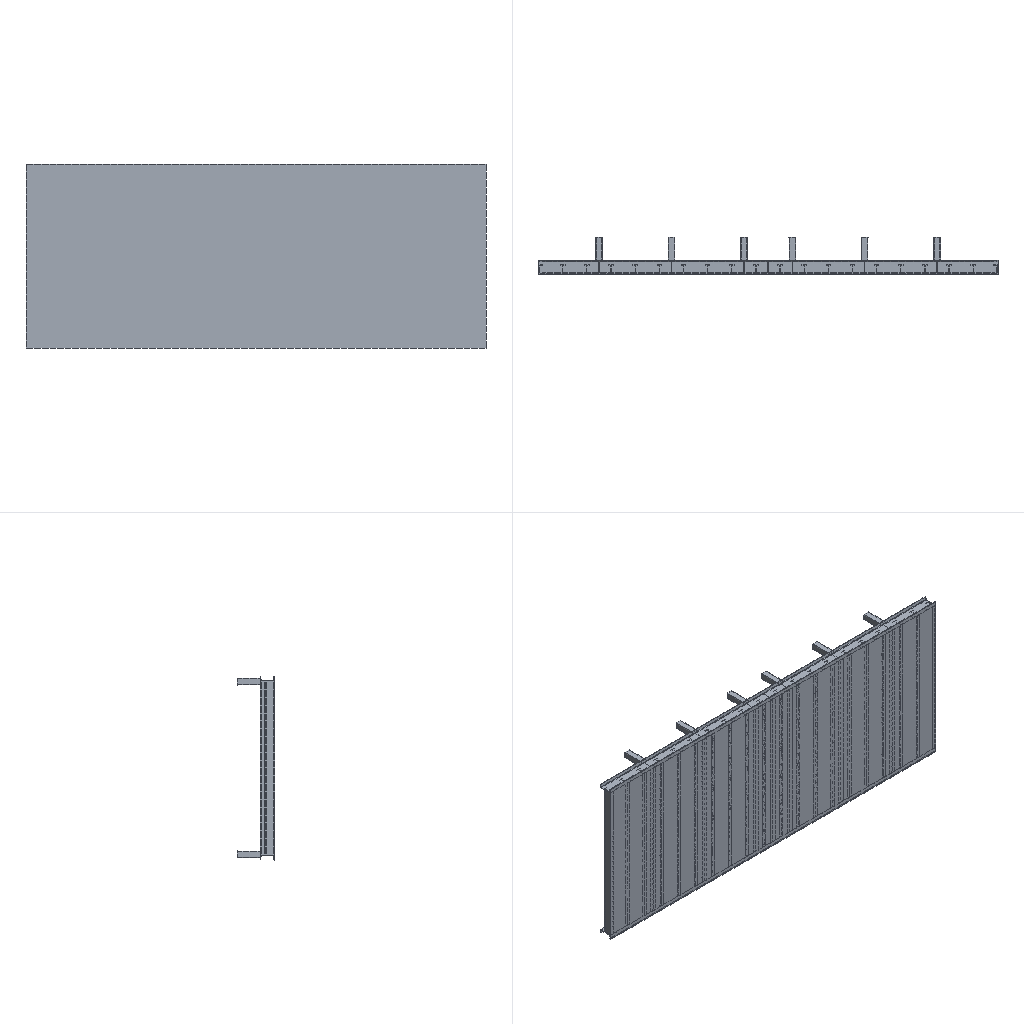Simulation study
Ansys APDL input file, long lists of numbers shortened:
/batch
/config,noeldb,1     ! force off writing results to database
*get,_wallstrt,active,,time,wall
! ANSYS input file written by Workbench version 2022 R1
! File used for geometry attach: F:\ansys（分析文件汇总)\结构件有限元分析qqww\fangan2_asm.STEP
/title,11--____ (E5)
! ****** Begin Custom Load Command Snippet ******
/COM, ACT Extensions:
/COM,     LSDYNA, 2021.1
/COM,
! ****** End   Custom Load Command Snippet ******
*DIM,_wb_ProjectScratch_dir,string,248
_wb_ProjectScratch_dir(1) = 'F:\ansys（分析文件汇总)\结构件有限元分析qqww\_ProjectScratch\Scr0353\'
*DIM,_wb_SolverFiles_dir,string,248
_wb_SolverFiles_dir(1) = 'F:\ansys（分析文件汇总)\结构件有限元分析qqww\11_files\dp0\SYS-2\MECH\'
*DIM,_wb_userfiles_dir,string,248
_wb_userfiles_dir(1) = 'F:\ansys（分析文件汇总)\结构件有限元分析qqww\11_files\user_files\'
/com,--- Data in consistent NMM units. See Solving Units in the help system for more information.
/units,MPA
/nopr
/wb,file,start              !  signify a WB generated input file
/prep7
! Turn off shape checking because checks already performed inside WB mesher.
! See help system for more information.
SHPP,OFF,,NOWARN
/nolist
etcon,set             ! allow ANSYS to choose best KEYOP's for 180x elements, resets any applicable keyopt to MAPDL defaults
/com,*********** Nodes for the whole assembly ***********
nblock,3,,254075
(1i9,3e20.9e3)
        1    -2.028857864E+03     3.100000000E+02     1.805857864E+03
! (230977 more lines like these left out)
-1
/wb,elem,start            !  set before creation of elements
/com,*********** Elements for Body 1 "1040MUTAI_ASM|1040MUTAI-1|1040MUTAI-1[1]" ***********
et,1,187
eblock,19,solid,,24586
(19i9)
        1        1        1        1        0        0        0        0       10        0      961    11084    14484    13060    15242    40608    51091    40606    40609
! (49171 more lines like these left out)
-1
/com,*********** Elements for Body 2 "1040MUTAI_ASM|1040MUTAI-2|1040MUTAI-2[1]" ***********
et,2,187
eblock,19,solid,,3615
(19i9)
        2        2        2        2        0        0        0        0       10        0    51948   109960   109998   109997   110036   112452   112614   112451   112454
! (7229 more lines like these left out)
-1
/com,*********** Elements for Body 3 "1040MUTAI_ASM|1040MUTAI-2|1040MUTAI-2[1][2]" ***********
et,3,187
eblock,19,solid,,3615
(19i9)
        3        3        3        3        0        0        0        0       10        0    44718    96224    96262    96261    96300    98716    98878    98715    98718
! (7229 more lines like these left out)
-1
/com,*********** Elements for Body 4 "1040MUTAI_ASM|1040MUTAI-2|1040MUTAI-2[1][3]" ***********
et,4,187
eblock,19,solid,,3615
(19i9)
        4        4        4        4        0        0        0        0       10        0    66408   137432   137470   137469   137508   139924   140086   139923   139926
! (7229 more lines like these left out)
-1
/com,*********** Elements for Body 5 "1040MUTAI_ASM|1040MUTAI-2|1040MUTAI-2[1][4]" ***********
et,5,187
eblock,19,solid,,3615
(19i9)
        5        5        5        5        0        0        0        0       10        0    33873    75620    75658    75657    75696    78112    78274    78111    78114
! (7229 more lines like these left out)
-1
! (37 more sections like these left out)
/wb,elem,end               !  done creating elements
/com,*********** Send User Defined Coordinate System(s) ***********
csys,0
toffst,273.15,  ! Temperature offset from absolute zero
/com,*********** Set Reference Temperature ***********
tref,22.
/wb,mat,start              !  starting to send materials
/com,*********** Send Materials ***********
Temperature = 'TEMP' ! Temperature
MP,DENS,1,7.85e-09,	! tonne mm^-3
MP,ALPX,1,1.2e-05,	! C^-1
MP,C,1,434000000,	! mm^2 s^-2 C^-1
MP,KXX,1,60.5,	! tonne mm s^-3 C^-1
MP,RSVX,1,0.00017,	! ohm mm
MP,EX,1,200000,	! tonne s^-2 mm^-1
MP,NUXY,1,0.3,
MP,MURX,1,10000,
Temperature = 'TEMP' ! Temperature
MP,DENS,2,7.85e-09,	! tonne mm^-3
MP,ALPX,2,1.2e-05,	! C^-1
MP,C,2,434000000,	! mm^2 s^-2 C^-1
MP,KXX,2,60.5,	! tonne mm s^-3 C^-1
MP,RSVX,2,0.00017,	! ohm mm
MP,EX,2,200000,	! tonne s^-2 mm^-1
MP,NUXY,2,0.3,
MP,MURX,2,10000,
Temperature = 'TEMP' ! Temperature
MP,DENS,3,7.85e-09,	! tonne mm^-3
MP,ALPX,3,1.2e-05,	! C^-1
MP,C,3,434000000,	! mm^2 s^-2 C^-1
MP,KXX,3,60.5,	! tonne mm s^-3 C^-1
MP,RSVX,3,0.00017,	! ohm mm
MP,EX,3,200000,	! tonne s^-2 mm^-1
MP,NUXY,3,0.3,
MP,MURX,3,10000,
Temperature = 'TEMP' ! Temperature
MP,DENS,4,7.85e-09,	! tonne mm^-3
MP,ALPX,4,1.2e-05,	! C^-1
MP,C,4,434000000,	! mm^2 s^-2 C^-1
MP,KXX,4,60.5,	! tonne mm s^-3 C^-1
MP,RSVX,4,0.00017,	! ohm mm
MP,EX,4,200000,	! tonne s^-2 mm^-1
MP,NUXY,4,0.3,
MP,MURX,4,10000,
Temperature = 'TEMP' ! Temperature
MP,DENS,5,7.85e-09,	! tonne mm^-3
MP,ALPX,5,1.2e-05,	! C^-1
MP,C,5,434000000,	! mm^2 s^-2 C^-1
MP,KXX,5,60.5,	! tonne mm s^-3 C^-1
MP,RSVX,5,0.00017,	! ohm mm
MP,EX,5,200000,	! tonne s^-2 mm^-1
MP,NUXY,5,0.3,
MP,MURX,5,10000,
Temperature = 'TEMP' ! Temperature
MP,DENS,6,7.85e-09,	! tonne mm^-3
MP,ALPX,6,1.2e-05,	! C^-1
MP,C,6,434000000,	! mm^2 s^-2 C^-1
MP,KXX,6,60.5,	! tonne mm s^-3 C^-1
MP,RSVX,6,0.00017,	! ohm mm
MP,EX,6,200000,	! tonne s^-2 mm^-1
MP,NUXY,6,0.3,
MP,MURX,6,10000,
Temperature = 'TEMP' ! Temperature
MP,DENS,7,7.85e-09,	! tonne mm^-3
MP,ALPX,7,1.2e-05,	! C^-1
MP,C,7,434000000,	! mm^2 s^-2 C^-1
MP,KXX,7,60.5,	! tonne mm s^-3 C^-1
MP,RSVX,7,0.00017,	! ohm mm
MP,EX,7,200000,	! tonne s^-2 mm^-1
MP,NUXY,7,0.3,
MP,MURX,7,10000,
Temperature = 'TEMP' ! Temperature
MP,DENS,8,7.85e-09,	! tonne mm^-3
MP,ALPX,8,1.2e-05,	! C^-1
MP,C,8,434000000,	! mm^2 s^-2 C^-1
MP,KXX,8,60.5,	! tonne mm s^-3 C^-1
MP,RSVX,8,0.00017,	! ohm mm
MP,EX,8,200000,	! tonne s^-2 mm^-1
MP,NUXY,8,0.3,
MP,MURX,8,10000,
Temperature = 'TEMP' ! Temperature
MP,DENS,9,7.85e-09,	! tonne mm^-3
MP,ALPX,9,1.2e-05,	! C^-1
MP,C,9,434000000,	! mm^2 s^-2 C^-1
MP,KXX,9,60.5,	! tonne mm s^-3 C^-1
MP,RSVX,9,0.00017,	! ohm mm
MP,EX,9,200000,	! tonne s^-2 mm^-1
! (299 more lines like these left out)
/wb,mat,end                !  done sending materials
!************************* Model Summary ********************
!1040MUTAI_ASM|1040MUTAI-1|1040MUTAI-1[1],	Q235,	matid,	1
!1040MUTAI_ASM|1040MUTAI-2|1040MUTAI-2[1],	Q235,	matid,	2
!1040MUTAI_ASM|1040MUTAI-2|1040MUTAI-2[1][2],	Q235,	matid,	3
! (41 more lines like these left out)
*get,_xmin,node,,mnloc,x
*get,_ymin,node,,mnloc,y
*get,_zmin,node,,mnloc,z
*get,_xmax,node,,mxloc,x
*get,_ymax,node,,mxloc,y
*get,_zmax,node,,mxloc,z
_ASMDIAG=(_xmax-_xmin)*(_xmax-_xmin)+(_ymax-_ymin)*(_ymax-_ymin)+(_zmax-_zmin)*(_zmax-_zmin)
_ASMDIAG=SQRT(_ASMDIAG)
/wb,contact,start          !  starting to send contact
/com,*********** Create Contact "接触区域" ***********
/com,            Real Constant Set For Above Contact Is 44 & 43
*set,tid,44
*set,cid,43
r,tid
r,cid
et,tid,170
et,cid,174
eblock,10,,,243
(15i9)
   173971       44       44       44        0    13244    14656    15577    15577    52001    56323    15577    52003
! (242 more lines like these left out)
-1
eblock,10,,,243
(15i9)
   174214       43       43       43        0    13244    14656    15577    15577    52001    56323    15577    52003
! (242 more lines like these left out)
-1
eblock,10,,,152
(15i9)
   174457       43       44       43        0   110820   109929   110843   110843   112209   112210   110843   116612
! (151 more lines like these left out)
-1
eblock,10,,,152
(15i9)
   174609       44       43       44        0   110820   109929   110843   110843   112209   112210   110843   116612
! (151 more lines like these left out)
-1
keyo,cid,8,2               ! auto create asymmetric contact (from Program Controlled setting)
keyo,cid,10,0              ! adjust contact stiffness each NR iteration (from Program Controlled setting)
keyo,cid,12,5              ! bonded always
keyo,cid,18,1              ! small sliding turned on by application
keyo,cid,2,0               ! augmented Lagrange (from Program Controlled setting)
keyo,cid,4,0               ! on Gauss point (from Program Controlled setting)
keyo,cid,9,1               ! ignore initial gaps/penetration
keyo,cid,7,0               ! No Prediction
rmod,tid,3,10.      ! FKN
rmod,tid,5,0.       ! ICONT
rmod,tid,6,0.       ! PINB
rmod,tid,10,0.      ! CNOF
rmod,tid,12,0.      ! FKT
rmod,tid,36,617     ! WB DSID
rmod,cid,3,10.      ! FKN
rmod,cid,5,0.       ! ICONT
rmod,cid,6,0.       ! PINB
rmod,cid,10,0.      ! CNOF
rmod,cid,12,0.      ! FKT
rmod,cid,36,617     ! WB DSID
/com,*********** Create Contact "接触区域 2" ***********
/com,            Real Constant Set For Above Contact Is 46 & 45
*set,tid,46
*set,cid,45
r,tid
r,cid
et,tid,170
et,cid,174
eblock,10,,,253
(15i9)
   174761       46       46       46        0    14570    15059    16027    16027    56183    56973    16027    56184
! (252 more lines like these left out)
-1
eblock,10,,,253
(15i9)
   175014       45       45       45        0    14570    15059    16027    16027    56183    56973    16027    56184
! (252 more lines like these left out)
-1
eblock,10,,,152
(15i9)
   175267       45       46       45        0    97084    96193    97107    97107    98473    98474    97107   102876
! (151 more lines like these left out)
-1
eblock,10,,,152
(15i9)
   175419       46       45       46        0    97084    96193    97107    97107    98473    98474    97107   102876
! (151 more lines like these left out)
-1
keyo,cid,8,2               ! auto create asymmetric contact (from Program Controlled setting)
keyo,cid,10,0              ! adjust contact stiffness each NR iteration (from Program Controlled setting)
keyo,cid,12,5              ! bonded always
keyo,cid,18,1              ! small sliding turned on by application
keyo,cid,2,0               ! augmented Lagrange (from Program Controlled setting)
keyo,cid,4,0               ! on Gauss point (from Program Controlled setting)
keyo,cid,9,1               ! ignore initial gaps/penetration
keyo,cid,7,0               ! No Prediction
rmod,tid,3,10.      ! FKN
rmod,tid,5,0.       ! ICONT
rmod,tid,6,0.       ! PINB
rmod,tid,10,0.      ! CNOF
rmod,tid,12,0.      ! FKT
rmod,tid,36,620     ! WB DSID
rmod,cid,3,10.      ! FKN
rmod,cid,5,0.       ! ICONT
rmod,cid,6,0.       ! PINB
rmod,cid,10,0.      ! CNOF
rmod,cid,12,0.      ! FKT
rmod,cid,36,620     ! WB DSID
/com,*********** Create Contact "接触区域 3" ***********
/com,            Real Constant Set For Above Contact Is 48 & 47
*set,tid,48
*set,cid,47
r,tid
r,cid
et,tid,170
et,cid,174
eblock,10,,,241
(15i9)
   175571       48       48       48        0    12403    14452    14310    14310    47331    55626    14310    47329
! (240 more lines like these left out)
-1
eblock,10,,,241
(15i9)
   175812       47       47       47        0    12403    14452    14310    14310    47331    55626    14310    47329
! (240 more lines like these left out)
-1
eblock,10,,,152
(15i9)
   176053       47       48       47        0   138292   137401   138315   138315   139681   139682   138315   144084
! (151 more lines like these left out)
-1
eblock,10,,,152
(15i9)
   176205       48       47       48        0   138292   137401   138315   138315   139681   139682   138315   144084
! (151 more lines like these left out)
-1
keyo,cid,8,2               ! auto create asymmetric contact (from Program Controlled setting)
keyo,cid,10,0              ! adjust contact stiffness each NR iteration (from Program Controlled setting)
keyo,cid,12,5              ! bonded always
keyo,cid,18,1              ! small sliding turned on by application
keyo,cid,2,0               ! augmented Lagrange (from Program Controlled setting)
keyo,cid,4,0               ! on Gauss point (from Program Controlled setting)
keyo,cid,9,1               ! ignore initial gaps/penetration
keyo,cid,7,0               ! No Prediction
rmod,tid,3,10.      ! FKN
rmod,tid,5,0.       ! ICONT
rmod,tid,6,0.       ! PINB
rmod,tid,10,0.      ! CNOF
rmod,tid,12,0.      ! FKT
rmod,tid,36,623     ! WB DSID
rmod,cid,3,10.      ! FKN
rmod,cid,5,0.       ! ICONT
rmod,cid,6,0.       ! PINB
rmod,cid,10,0.      ! CNOF
rmod,cid,12,0.      ! FKT
rmod,cid,36,623     ! WB DSID
/com,*********** Create Contact "接触区域 4" ***********
/com,            Real Constant Set For Above Contact Is 50 & 49
*set,tid,50
*set,cid,49
r,tid
r,cid
et,tid,170
et,cid,174
eblock,10,,,239
(15i9)
   176357       50       50       50        0    13090    13815    14619    14619    51233    54287    14619    51236
! (238 more lines like these left out)
-1
eblock,10,,,239
(15i9)
   176596       49       49       49        0    13090    13815    14619    14619    51233    54287    14619    51236
! (238 more lines like these left out)
-1
eblock,10,,,152
(15i9)
   176835       49       50       49        0    76480    75589    76503    76503    77869    77870    76503    82272
! (151 more lines like these left out)
-1
eblock,10,,,152
(15i9)
   176987       50       49       50        0    76480    75589    76503    76503    77869    77870    76503    82272
! (151 more lines like these left out)
-1
keyo,cid,8,2               ! auto create asymmetric contact (from Program Controlled setting)
keyo,cid,10,0              ! adjust contact stiffness each NR iteration (from Program Controlled setting)
keyo,cid,12,5              ! bonded always
keyo,cid,18,1              ! small sliding turned on by application
keyo,cid,2,0               ! augmented Lagrange (from Program Controlled setting)
keyo,cid,4,0               ! on Gauss point (from Program Controlled setting)
keyo,cid,9,1               ! ignore initial gaps/penetration
keyo,cid,7,0               ! No Prediction
rmod,tid,3,10.      ! FKN
rmod,tid,5,0.       ! ICONT
rmod,tid,6,0.       ! PINB
rmod,tid,10,0.      ! CNOF
rmod,tid,12,0.      ! FKT
rmod,tid,36,626     ! WB DSID
rmod,cid,3,10.      ! FKN
rmod,cid,5,0.       ! ICONT
rmod,cid,6,0.       ! PINB
rmod,cid,10,0.      ! CNOF
rmod,cid,12,0.      ! FKT
rmod,cid,36,626     ! WB DSID
/com,*********** Create Contact "接触区域 5" ***********
/com,            Real Constant Set For Above Contact Is 52 & 51
*set,tid,52
*set,cid,51
r,tid
r,cid
et,tid,170
et,cid,174
eblock,10,,,275
(15i9)
   177139       52       52       52        0    15557    15830    15747    15747    57464    57559    15747    57463
! (274 more lines like these left out)
-1
eblock,10,,,275
(15i9)
   177414       51       51       51        0    15557    15830    15747    15747    57464    57559    15747    57463
! (274 more lines like these left out)
-1
eblock,10,,,152
(15i9)
   177689       51       52       51        0    90216    89325    90239    90239    91605    91606    90239    96008
! (151 more lines like these left out)
-1
eblock,10,,,152
(15i9)
   177841       52       51       52        0    90216    89325    90239    90239    91605    91606    90239    96008
! (151 more lines like these left out)
-1
keyo,cid,8,2               ! auto create asymmetric contact (from Program Controlled setting)
keyo,cid,10,0              ! adjust contact stiffness each NR iteration (from Program Controlled setting)
keyo,cid,12,5              ! bonded always
keyo,cid,18,1              ! small sliding turned on by application
keyo,cid,2,0               ! augmented Lagrange (from Program Controlled setting)
keyo,cid,4,0               ! on Gauss point (from Program Controlled setting)
keyo,cid,9,1               ! ignore initial gaps/penetration
keyo,cid,7,0               ! No Prediction
rmod,tid,3,10.      ! FKN
rmod,tid,5,0.       ! ICONT
rmod,tid,6,0.       ! PINB
rmod,tid,10,0.      ! CNOF
rmod,tid,12,0.      ! FKT
rmod,tid,36,629     ! WB DSID
rmod,cid,3,10.      ! FKN
rmod,cid,5,0.       ! ICONT
rmod,cid,6,0.       ! PINB
rmod,cid,10,0.      ! CNOF
rmod,cid,12,0.      ! FKT
rmod,cid,36,629     ! WB DSID
! (102 more sections like these left out)
/wb,contact,end            !  done creating contacts
/golist
/wb,load,start             !  starting to send loads
/com,*********** Fixed Supports ***********
CMBLOCK,_FIXEDSU,NODE,      960
(8i10)
        37        38        39        52        53        62        63        72
! (119 more lines like these left out)
cmsel,s,_FIXEDSU
d,all,all
nsel,all
/com,*********** Define Force Using Surface Effect Elements ***********
local,12,0,0.,0.,0.,0.,0.,0.
csys,0
et,257,154
eblock,10,,,918
(15i9)
   202211      257      257      257       12     8392     8393     8755     8755    21860    21871     8755    21861
! (917 more lines like these left out)
-1
esel,s,type,,257
keyop,257,2,1                ! Apply load in local coordinate system
keyop,257,7,1                ! Use original area so load is constant in large deformation
esel,all
/com,*********** Define Force Using Surface Effect Elements ***********
local,13,0,0.,0.,0.,0.,0.,0.
csys,0
et,258,154
eblock,10,,,218
(15i9)
   203129      258      258      258       13     9917     9938     9926     9926    30786    30845     9926    30785
! (217 more lines like these left out)
-1
esel,s,type,,258
keyop,258,2,1                ! Apply load in local coordinate system
keyop,258,7,1                ! Use original area so load is constant in large deformation
esel,all
/gst,on,on
fini
*get,_numnode,node,0,count
*get,_numelem,elem,0,count
*get, _MAXELEMNUM, elem, 0, NUM, MAX
*get, _MAXNODENUM, node, 0, NUM, MAX
*get, _MAXELEMTYPE, etyp, 0, NUM, MAX
*get, _MAXREALCONST, real, 0, NUM, MAX
/go
/wb,load,end               !  done creating loads
/com,--- Number of total nodes = %_numnode%
/com,--- Number of contact elements = 29376
/com,--- Number of spring elements = 0
/com,--- Number of bearing elements = 0
/com,--- Number of solid elements = 104414
/com,--- Number of condensed parts = 0
/com,--- Number of total elements = %_numelem%
*get,_wallbsol,active,,time,wall
/com,****************************************************************************
/com,*************************    SOLUTION       ********************************
/com,****************************************************************************
/solu
antype,0                   ! static analysis
_thickRatio=0.0476  ! Ratio of thick parts in the model
eqsl,sparse,,,,,1
cntr,print,1               ! print out contact info and also make no initial contact an error
cntr,out,yes               ! write contact output to file.cmn due to many contact pairs present
dmpoption,emat,no             ! Don't combine emat file for DANSYS
dmpoption,esav,no             ! Don't combine esav file for DANSYS
nldiag,cont,iter           ! print out contact info each equilibrium iteration
rescontrol,,none                 ! Do not keep any restart files
/com,****************************************************
/com,******************* SOLVE FOR LS 1 OF 1 ****************
esel,s,type,,257
nsle
sfe,all,1,pres,1,0.
sfe,all,2,pres,1,6.55725419664069e-002
sfe,all,3,pres,1,0.
esel,s,type,,258
nsle
sfe,all,1,pres,1,0.
sfe,all,2,pres,1,0.2083
sfe,all,3,pres,1,0.
nsel,all
esel,all
acel,0.,0.,9806.65
/nopr
/gopr
nsub,1,1,1
time,1.
outres,erase
outres,all,none
outres,nsol,all,
outres,rsol,all
outres,eangl,all
outres,etmp,all
outres,veng,all
outres,strs,all,
outres,epel,all,
outres,eppl,all,
outres,cont,all,
! *********** WB SOLVE COMMAND ***********
! check interactive state
*get,ANSINTER_,active,,int
*if,ANSINTER_,ne,0,then
/eof
*endif
solve
/com *************** Write FE CONNECTORS *********
CEWRITE,file,ce,,INTE
/com,****************************************************
/com,*************** FINISHED SOLVE FOR LS 1 *************
*get,_wallasol,active,,time,wall
/nopr
*get,_numnode,node,0,count
*get,_numelem,elem,0,count
*get, _MAXELEMNUM, elem, 0, NUM, MAX
*get, _MAXNODENUM, node, 0, NUM, MAX,,,INTERNAL
*get, _MAXELEMTYPE, etyp, 0, NUM, MAX
*get, _MAXREALCONST, real, 0, NUM, MAX
/gopr
/post1
xmlo,ENCODING,ISO-8859-1
xmlo,parm
/xml,parm,xml
fini
/gopr
*get,_walldone,active,,time,wall
_preptime=(_wallbsol-_wallstrt)*3600
_solvtime=(_wallasol-_wallbsol)*3600
_posttime=(_walldone-_wallasol)*3600
_totaltim=(_walldone-_wallstrt)*3600
*get,_dlbratio,active,0,solu,dlbr
*get,_combtime,active,0,solu,comb
*get,_ssmode,active,0,solu,ssmm
*get,_ndofs,active,0,solu,ndof
*get,_sol_end_time,active,0,set,time
*if,_sol_end_time,eq,1.,then
/fclean				!clean distributed files
*endif
/com,--- Total number of nodes = %_numnode%
/com,--- Total number of elements = %_numelem%
/com,--- Element load balance ratio = %_dlbratio%
/com,--- Time to combine distributed files = %_combtime%
/com,--- Sparse memory mode = %_ssmode%
/com,--- Number of DOF = %_ndofs%
/wb,file,end               ! done with WB generated input